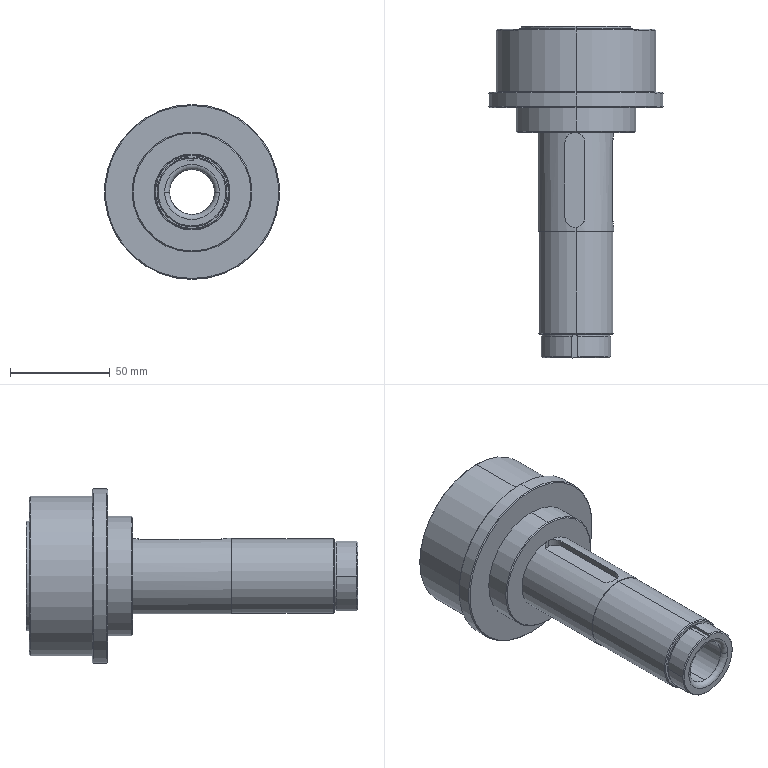Part | STEP file | 2026.6.15-Main Assembly图.sldasm-Part-158 | 1 solid | 92 faces | box 87.5 x 166 x 87.5 mm | volume 296087 mm3 | cylinder 41 | plane 28 | cone 11 | spline 8 | torus 4 | commonest cylinder face diameters 5 x20 34 x3 35 x3 38 x3 22.5 x2 37.5 x2